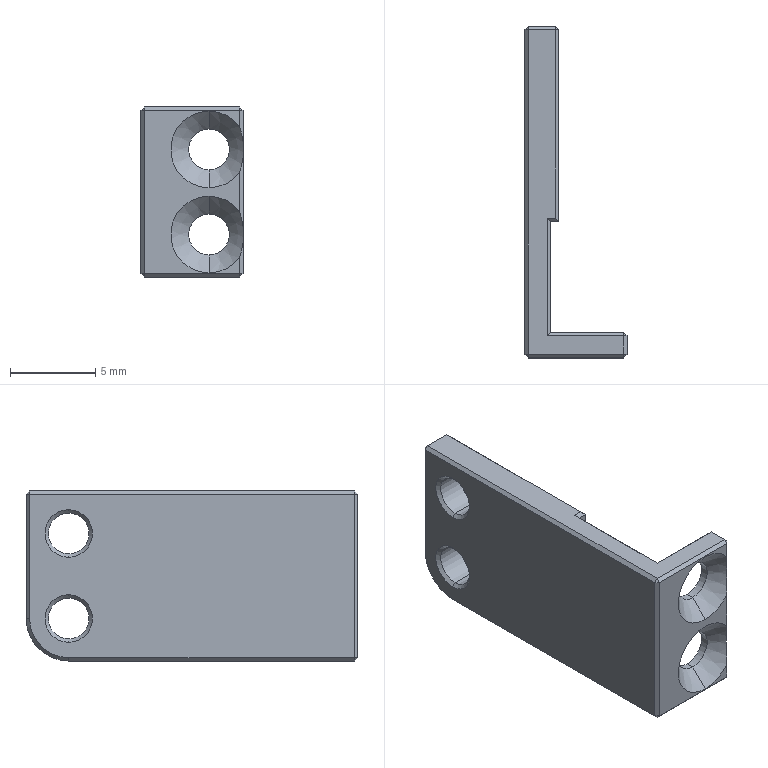Part | SolidWorks | features ICE 3, Chamfer 1, Extrusion 1, Fillet 1, HoleWzd 1 | 1 solid | 63 faces | box 6 x 19.5 x 10 mm | volume 368.969 mm3 | plane 40 | cone 14 | cylinder 9 | commonest cylinder face diameters 2.4 x8 5 x1